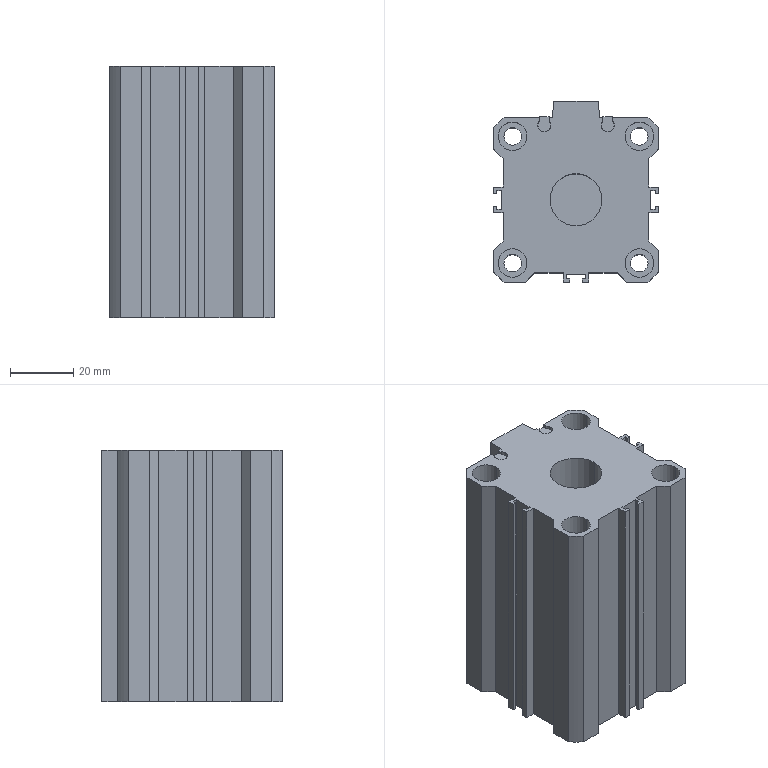Part | STEP file | bA_CDQ2B40_40DM_M9N_0_ | 1 solid | 145 faces | box 52 x 57 x 79.5 mm | volume 176566 mm3 | plane 91 | cylinder 50 | cone 4 | commonest cylinder face diameters 9 x16 5.5 x8 4 x6 4.2 x6 2.7 x4 8.57 x4